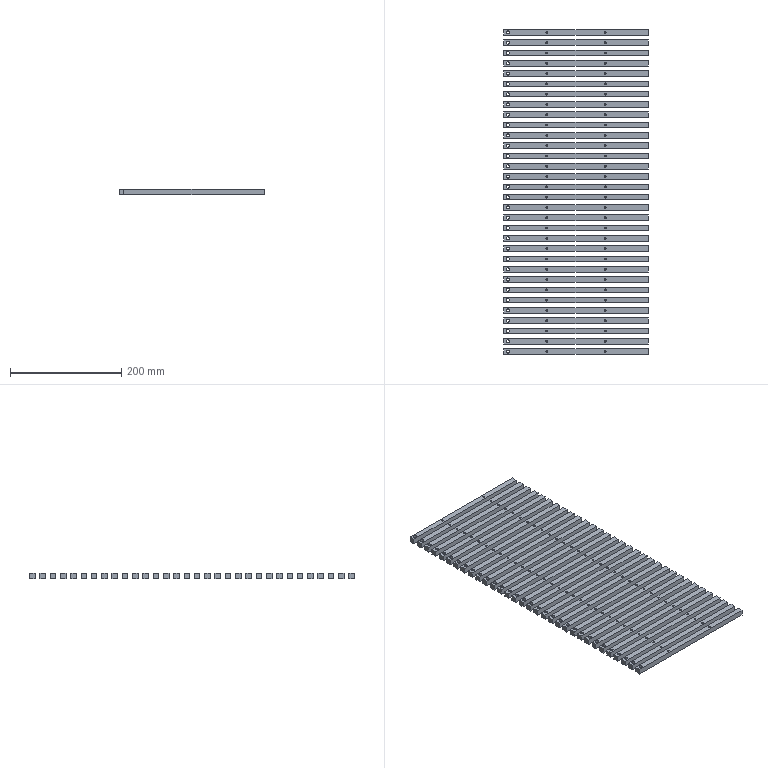Part | 32 solids | 512 faces | box 260 x 583.5 x 10 mm | volume 816069 mm3 | cylinder 256 | plane 192 | cone 64 | commonest cylinder face diameters 3.3 x192 5.5 x64